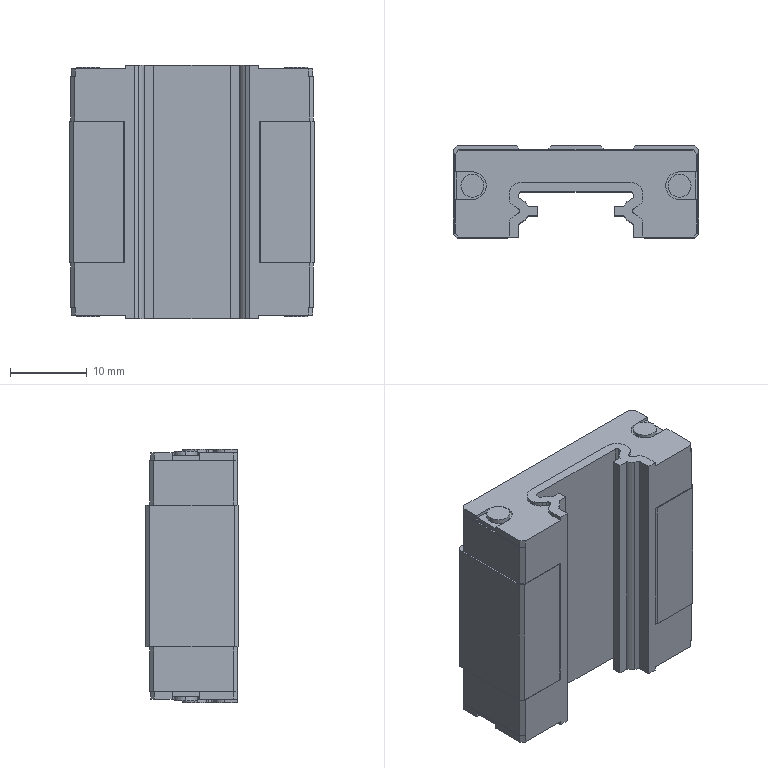Part | SolidWorks | 1 solid | 163 faces | box 32 x 12 x 33.1 mm | volume 9311 mm3 | plane 117 | cylinder 42 | cone 4 | commonest cylinder face diameters 3 x10 2.6 x8 0.8 x6 3.6 x6 2.5 x4 3.2 x4